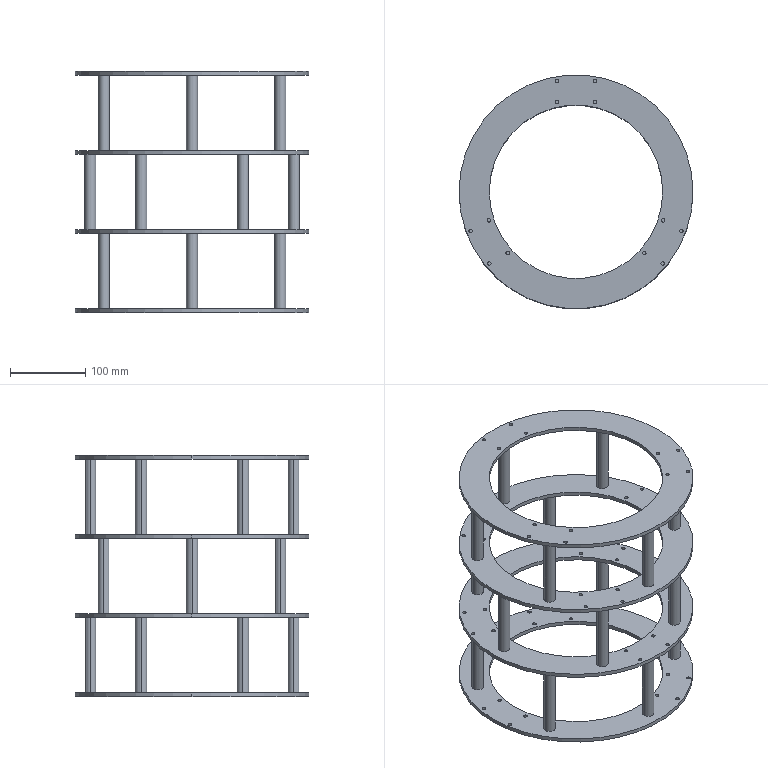Part | STEP file | Cutter head | 1 solid | 156 faces | box 310 x 310 x 320 mm | volume 992722 mm3 | cylinder 148 | plane 8 | commonest cylinder face diameters 4.5 x72 15 x36 4.8 x24 230 x8 310 x8